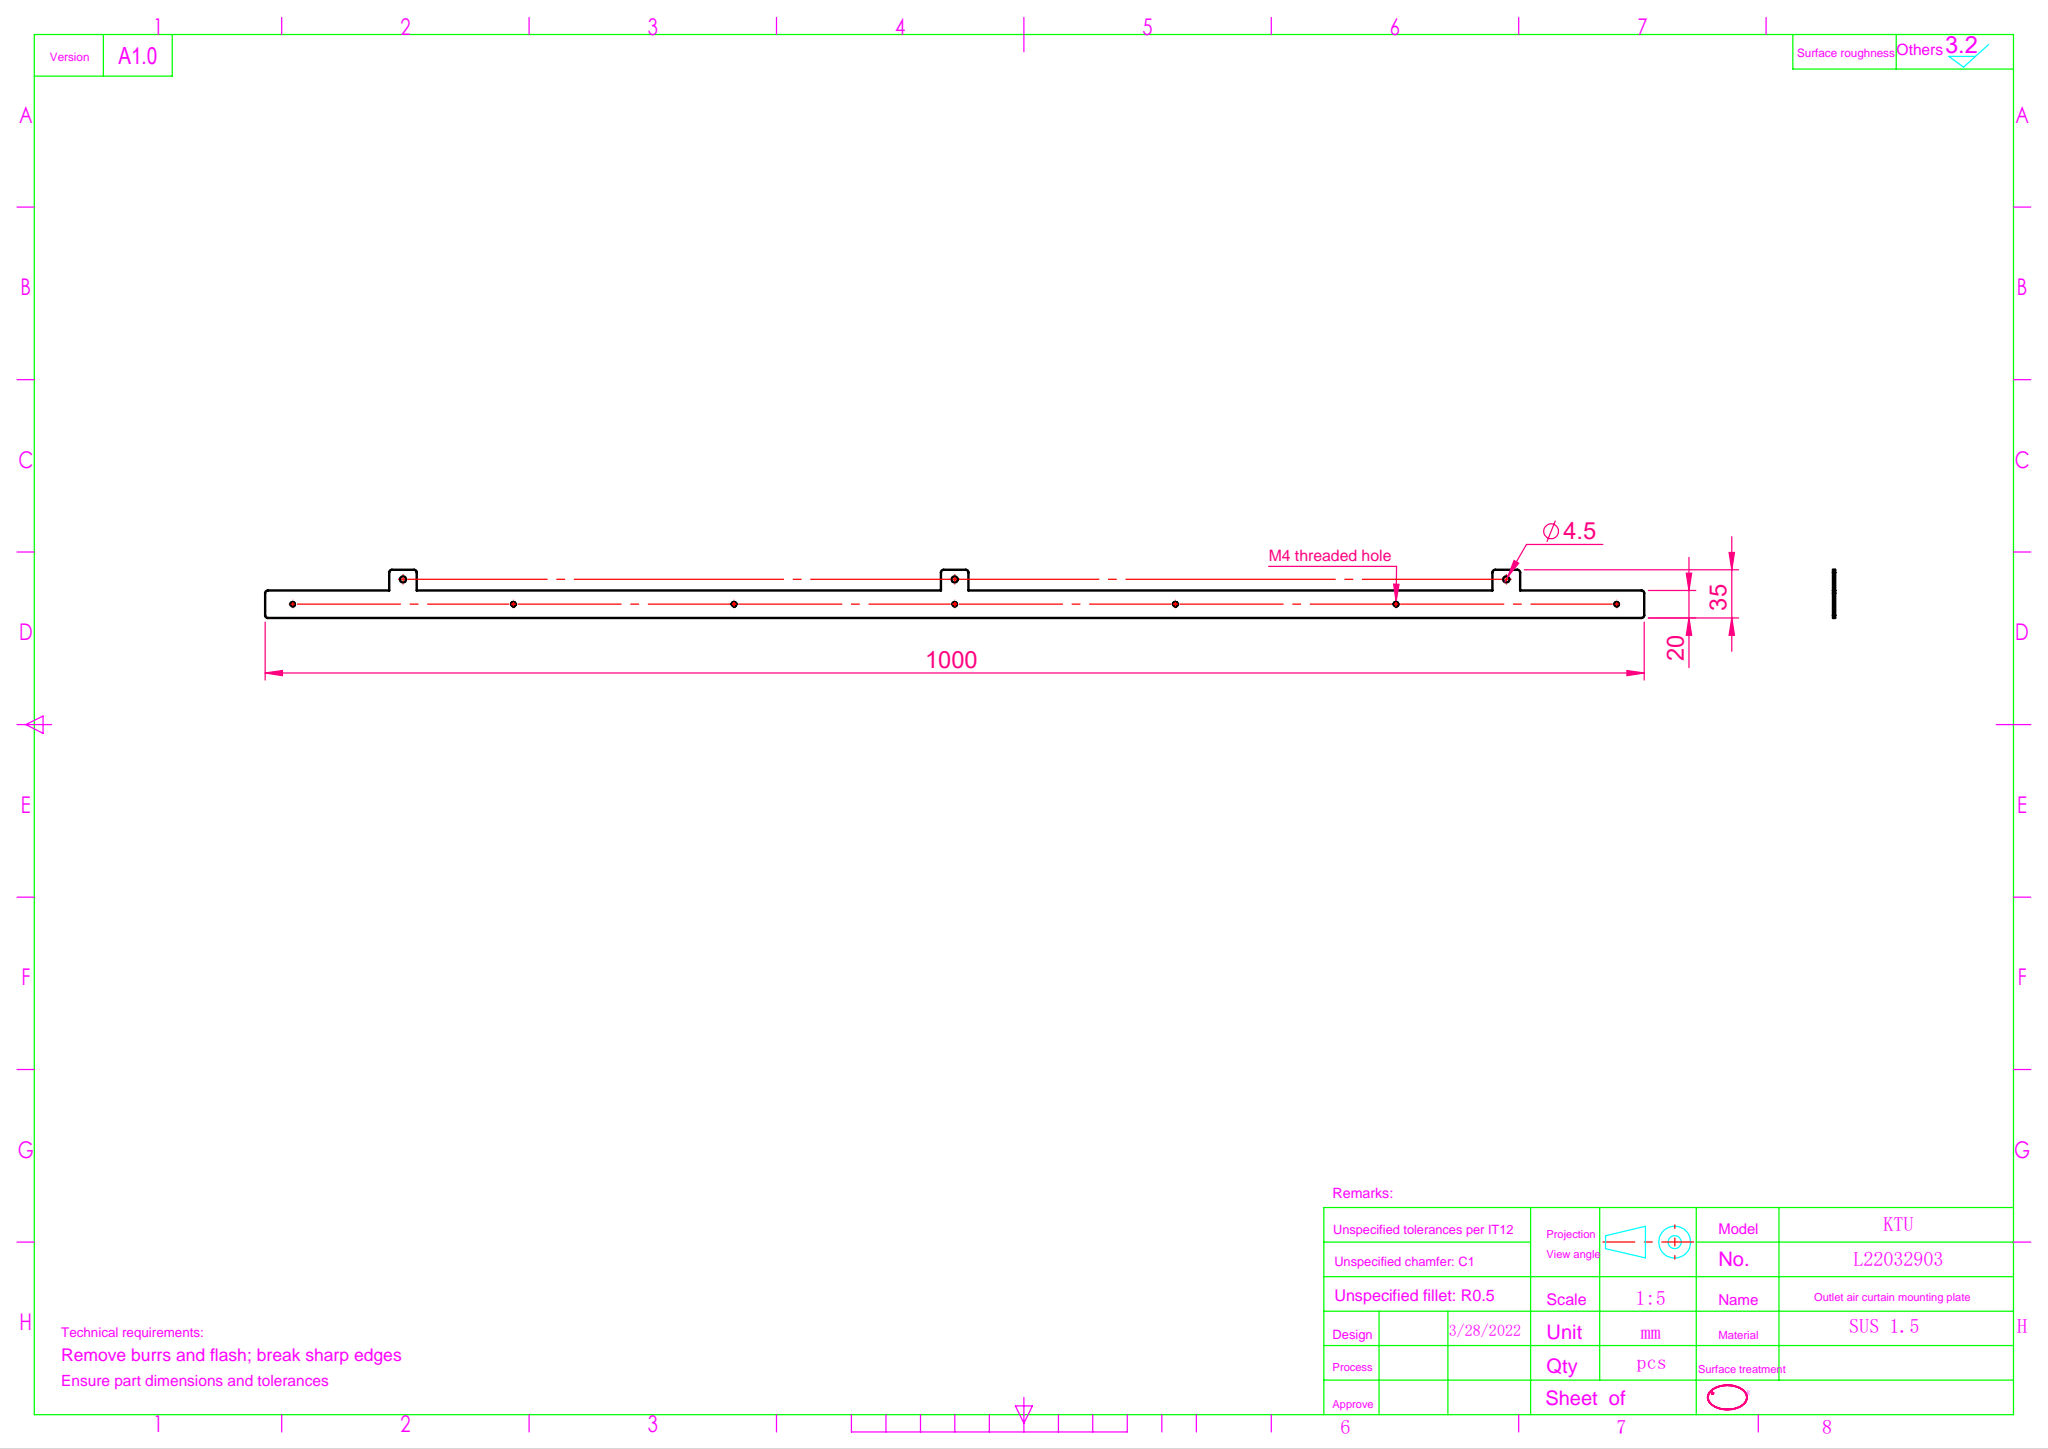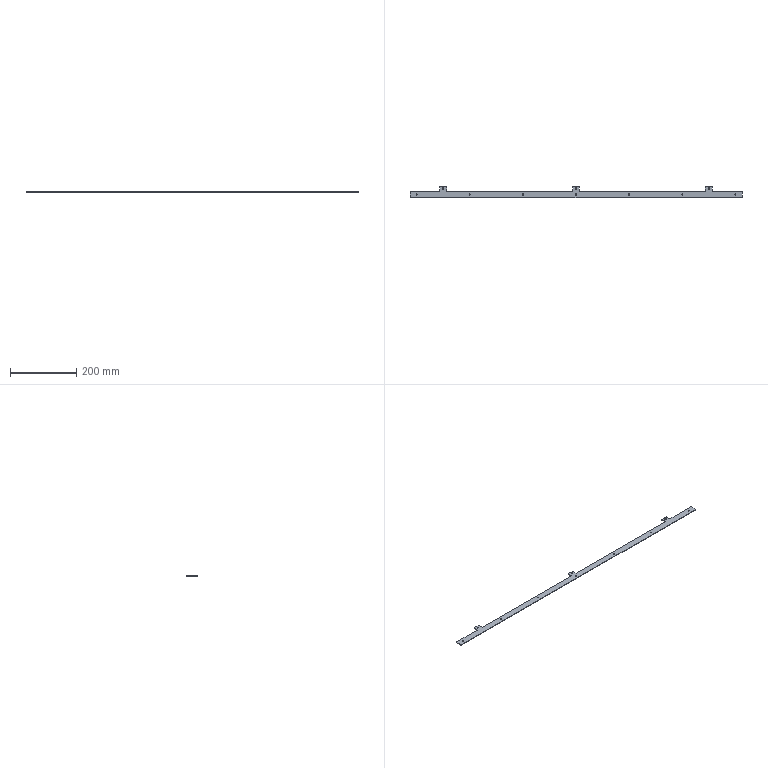Part | SolidWorks | features LPattern 2, SMBaseFlange 2, Fillet 1, FlatPattern 1, HoleWzd 1, ICE 1, SheetMetal 1 | 1 solid | 48 faces | box 1000 x 35 x 1.5 mm | volume 31176 mm3 | cylinder 30 | plane 18 | commonest cylinder face diameters 3.3 x14 4 x10 4.5 x6